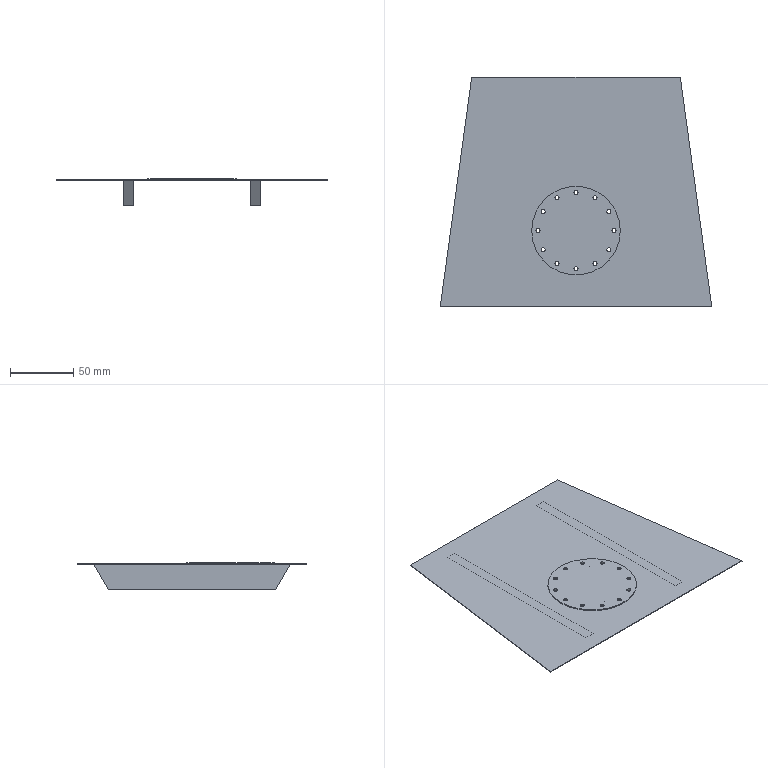Part | SolidWorks | features BaseBody 1 | 1 solid | 46 faces | box 214.2 x 181 x 21.3 mm | volume 65017 mm3 | cylinder 28 | plane 18 | commonest cylinder face diameters 3.2 x24 50 x2 70 x2
STEP:
#1=CARTESIAN_POINT('',(-16.6,85.981,1.3));
#2=VERTEX_POINT('',#1);
#3=CARTESIAN_POINT('',(-13.4,85.981,1.3));
#4=VERTEX_POINT('',#3);
#5=CARTESIAN_POINT('',(-15.,85.981,1.3));
#6=DIRECTION('',(0.,0.,1.));
#7=DIRECTION('',(-1.,0.,0.));
#8=AXIS2_PLACEMENT_3D('',#5,#6,#7);
#9=CIRCLE('',#8,1.6);
#10=EDGE_CURVE('',#2,#4,#9,.T.);
#11=ORIENTED_EDGE('',*,*,#10,.T.);
#12=CARTESIAN_POINT('',(-13.4,85.981,0.));
#13=VERTEX_POINT('',#12);
#14=CARTESIAN_POINT('',(-13.4,85.981,1.3));
#15=DIRECTION('',(0.,0.,-1.));
#16=VECTOR('',#15,1000.);
#17=LINE('',#14,#16);
#18=EDGE_CURVE('',#4,#13,#17,.T.);
#19=ORIENTED_EDGE('',*,*,#18,.T.);
#20=CARTESIAN_POINT('',(-16.6,85.981,0.));
#21=VERTEX_POINT('',#20);
#22=CARTESIAN_POINT('',(-15.,85.981,0.));
#23=DIRECTION('',(0.,0.,-1.));
#24=DIRECTION('',(-1.,0.,0.));
#25=AXIS2_PLACEMENT_3D('',#22,#23,#24);
#26=CIRCLE('',#25,1.6);
#27=EDGE_CURVE('',#13,#21,#26,.T.);
#28=ORIENTED_EDGE('',*,*,#27,.T.);
#29=CARTESIAN_POINT('',(-16.6,85.981,1.3));
#30=DIRECTION('',(0.,0.,-1.));
#31=VECTOR('',#30,1000.);
#32=LINE('',#29,#31);
#33=EDGE_CURVE('',#2,#21,#32,.T.);
#34=ORIENTED_EDGE('',*,*,#33,.F.);
#35=EDGE_LOOP('',(#11,#19,#28,#34));
#36=FACE_OUTER_BOUND('',#35,.T.);
#37=CARTESIAN_POINT('',(-15.,85.981,1.3));
#38=DIRECTION('',(0.,0.,-1.));
#39=DIRECTION('',(-1.,0.,0.));
#40=AXIS2_PLACEMENT_3D('',#37,#38,#39);
#41=CYLINDRICAL_SURFACE('',#40,1.6);
#42=ADVANCED_FACE('',(#36),#41,.F.);
#43=CARTESIAN_POINT('',(-25.,60.,0.5));
#44=VERTEX_POINT('',#43);
#45=CARTESIAN_POINT('',(25.,60.,0.5));
#46=VERTEX_POINT('',#45);
#47=CARTESIAN_POINT('',(0.,60.,0.5));
#48=DIRECTION('',(0.,0.,1.));
#49=DIRECTION('',(-1.,0.,0.));
#50=AXIS2_PLACEMENT_3D('',#47,#48,#49);
#51=CIRCLE('',#50,25.);
#52=EDGE_CURVE('',#44,#46,#51,.T.);
#53=ORIENTED_EDGE('',*,*,#52,.T.);
#54=CARTESIAN_POINT('',(25.,60.,0.));
#55=VERTEX_POINT('',#54);
#56=CARTESIAN_POINT('',(25.,60.,0.5));
#57=DIRECTION('',(0.,0.,-1.));
#58=VECTOR('',#57,1000.);
#59=LINE('',#56,#58);
#60=EDGE_CURVE('',#46,#55,#59,.T.);
#61=ORIENTED_EDGE('',*,*,#60,.T.);
#62=CARTESIAN_POINT('',(-25.,60.,0.));
#63=VERTEX_POINT('',#62);
#64=CARTESIAN_POINT('',(0.,60.,0.));
#65=DIRECTION('',(0.,0.,-1.));
#66=DIRECTION('',(-1.,0.,0.));
#67=AXIS2_PLACEMENT_3D('',#64,#65,#66);
#68=CIRCLE('',#67,25.);
#69=EDGE_CURVE('',#55,#63,#68,.T.);
#70=ORIENTED_EDGE('',*,*,#69,.T.);
#71=CARTESIAN_POINT('',(-25.,60.,0.5));
#72=DIRECTION('',(0.,0.,-1.));
#73=VECTOR('',#72,1000.);
#74=LINE('',#71,#73);
#75=EDGE_CURVE('',#44,#63,#74,.T.);
#76=ORIENTED_EDGE('',*,*,#75,.F.);
#77=EDGE_LOOP('',(#53,#61,#70,#76));
#78=FACE_OUTER_BOUND('',#77,.T.);
#79=CARTESIAN_POINT('',(0.,60.,0.5));
#80=DIRECTION('',(0.,0.,-1.));
#81=DIRECTION('',(-1.,0.,0.));
#82=AXIS2_PLACEMENT_3D('',#79,#80,#81);
#83=CYLINDRICAL_SURFACE('',#82,25.);
#84=ADVANCED_FACE('',(#78),#83,.F.);
#85=CARTESIAN_POINT('',(-24.381,45.,1.3));
#86=VERTEX_POINT('',#85);
#87=CARTESIAN_POINT('',(-27.581,45.,1.3));
#88=VERTEX_POINT('',#87);
#89=CARTESIAN_POINT('',(-25.981,45.,1.3));
#90=DIRECTION('',(0.,0.,-1.));
#91=DIRECTION('',(-1.,0.,0.));
#92=AXIS2_PLACEMENT_3D('',#89,#90,#91);
#93=CIRCLE('',#92,1.6);
#94=EDGE_CURVE('',#86,#88,#93,.T.);
#95=ORIENTED_EDGE('',*,*,#94,.F.);
#96=CARTESIAN_POINT('',(-24.381,45.,0.));
#97=VERTEX_POINT('',#96);
#98=CARTESIAN_POINT('',(-24.381,45.,1.3));
#99=DIRECTION('',(0.,0.,-1.));
#100=VECTOR('',#99,1000.);
#101=LINE('',#98,#100);
#102=EDGE_CURVE('',#86,#97,#101,.T.);
#103=ORIENTED_EDGE('',*,*,#102,.T.);
#104=CARTESIAN_POINT('',(-27.581,45.,0.));
#105=VERTEX_POINT('',#104);
#106=CARTESIAN_POINT('',(-25.981,45.,0.));
#107=DIRECTION('',(0.,0.,-1.));
#108=DIRECTION('',(-1.,0.,0.));
#109=AXIS2_PLACEMENT_3D('',#106,#107,#108);
#110=CIRCLE('',#109,1.6);
#111=EDGE_CURVE('',#97,#105,#110,.T.);
#112=ORIENTED_EDGE('',*,*,#111,.T.);
#113=CARTESIAN_POINT('',(-27.581,45.,1.3));
#114=DIRECTION('',(0.,0.,-1.));
#115=VECTOR('',#114,1000.);
#116=LINE('',#113,#115);
#117=EDGE_CURVE('',#88,#105,#116,.T.);
#118=ORIENTED_EDGE('',*,*,#117,.F.);
#119=EDGE_LOOP('',(#95,#103,#112,#118));
#120=FACE_OUTER_BOUND('',#119,.T.);
#121=CARTESIAN_POINT('',(-25.981,45.,1.3));
#122=DIRECTION('',(0.,0.,-1.));
#123=DIRECTION('',(-1.,0.,0.));
#124=AXIS2_PLACEMENT_3D('',#121,#122,#123);
#125=CYLINDRICAL_SURFACE('',#124,1.6);
#126=ADVANCED_FACE('',(#120),#125,.F.);
#127=CARTESIAN_POINT('',(-13.4,34.019,1.3));
#128=VERTEX_POINT('',#127);
#129=CARTESIAN_POINT('',(-16.6,34.019,1.3));
#130=VERTEX_POINT('',#129);
#131=CARTESIAN_POINT('',(-15.,34.019,1.3));
#132=DIRECTION('',(0.,0.,-1.));
#133=DIRECTION('',(-1.,0.,0.));
#134=AXIS2_PLACEMENT_3D('',#131,#132,#133);
#135=CIRCLE('',#134,1.6);
#136=EDGE_CURVE('',#128,#130,#135,.T.);
#137=ORIENTED_EDGE('',*,*,#136,.F.);
#138=CARTESIAN_POINT('',(-13.4,34.019,0.));
#139=VERTEX_POINT('',#138);
#140=CARTESIAN_POINT('',(-13.4,34.019,1.3));
#141=DIRECTION('',(0.,0.,-1.));
#142=VECTOR('',#141,1000.);
#143=LINE('',#140,#142);
#144=EDGE_CURVE('',#128,#139,#143,.T.);
#145=ORIENTED_EDGE('',*,*,#144,.T.);
#146=CARTESIAN_POINT('',(-16.6,34.019,0.));
#147=VERTEX_POINT('',#146);
#148=CARTESIAN_POINT('',(-15.,34.019,0.));
#149=DIRECTION('',(0.,0.,-1.));
#150=DIRECTION('',(-1.,0.,0.));
#151=AXIS2_PLACEMENT_3D('',#148,#149,#150);
#152=CIRCLE('',#151,1.6);
#153=EDGE_CURVE('',#139,#147,#152,.T.);
#154=ORIENTED_EDGE('',*,*,#153,.T.);
#155=CARTESIAN_POINT('',(-16.6,34.019,1.3));
#156=DIRECTION('',(0.,0.,-1.));
#157=VECTOR('',#156,1000.);
#158=LINE('',#155,#157);
#159=EDGE_CURVE('',#130,#147,#158,.T.);
#160=ORIENTED_EDGE('',*,*,#159,.F.);
#161=EDGE_LOOP('',(#137,#145,#154,#160));
#162=FACE_OUTER_BOUND('',#161,.T.);
#163=CARTESIAN_POINT('',(-15.,34.019,1.3));
#164=DIRECTION('',(0.,0.,-1.));
#165=DIRECTION('',(-1.,0.,0.));
#166=AXIS2_PLACEMENT_3D('',#163,#164,#165);
#167=CYLINDRICAL_SURFACE('',#166,1.6);
#168=ADVANCED_FACE('',(#162),#167,.F.);
#169=CARTESIAN_POINT('',(1.6,30.,1.3));
#170=VERTEX_POINT('',#169);
#171=CARTESIAN_POINT('',(-1.6,30.,1.3));
#172=VERTEX_POINT('',#171);
#173=CARTESIAN_POINT('',(0.,30.,1.3));
#174=DIRECTION('',(0.,0.,-1.));
#175=DIRECTION('',(-1.,0.,0.));
#176=AXIS2_PLACEMENT_3D('',#173,#174,#175);
#177=CIRCLE('',#176,1.6);
#178=EDGE_CURVE('',#170,#172,#177,.T.);
#179=ORIENTED_EDGE('',*,*,#178,.F.);
#180=CARTESIAN_POINT('',(1.6,30.,0.));
#181=VERTEX_POINT('',#180);
#182=CARTESIAN_POINT('',(1.6,30.,1.3));
#183=DIRECTION('',(0.,0.,-1.));
#184=VECTOR('',#183,1000.);
#185=LINE('',#182,#184);
#186=EDGE_CURVE('',#170,#181,#185,.T.);
#187=ORIENTED_EDGE('',*,*,#186,.T.);
#188=CARTESIAN_POINT('',(-1.6,30.,0.));
#189=VERTEX_POINT('',#188);
#190=CARTESIAN_POINT('',(0.,30.,0.));
#191=DIRECTION('',(0.,0.,-1.));
#192=DIRECTION('',(-1.,0.,0.));
#193=AXIS2_PLACEMENT_3D('',#190,#191,#192);
#194=CIRCLE('',#193,1.6);
#195=EDGE_CURVE('',#181,#189,#194,.T.);
#196=ORIENTED_EDGE('',*,*,#195,.T.);
#197=CARTESIAN_POINT('',(-1.6,30.,1.3));
#198=DIRECTION('',(0.,0.,-1.));
#199=VECTOR('',#198,1000.);
#200=LINE('',#197,#199);
#201=EDGE_CURVE('',#172,#189,#200,.T.);
#202=ORIENTED_EDGE('',*,*,#201,.F.);
#203=EDGE_LOOP('',(#179,#187,#196,#202));
#204=FACE_OUTER_BOUND('',#203,.T.);
#205=CARTESIAN_POINT('',(0.,30.,1.3));
#206=DIRECTION('',(0.,0.,-1.));
#207=DIRECTION('',(-1.,0.,0.));
#208=AXIS2_PLACEMENT_3D('',#205,#206,#207);
#209=CYLINDRICAL_SURFACE('',#208,1.6);
#210=ADVANCED_FACE('',(#204),#209,.F.);
#211=CARTESIAN_POINT('',(16.6,34.019,1.3));
#212=VERTEX_POINT('',#211);
#213=CARTESIAN_POINT('',(13.4,34.019,1.3));
#214=VERTEX_POINT('',#213);
#215=CARTESIAN_POINT('',(15.,34.019,1.3));
#216=DIRECTION('',(0.,0.,-1.));
#217=DIRECTION('',(-1.,0.,0.));
#218=AXIS2_PLACEMENT_3D('',#215,#216,#217);
#219=CIRCLE('',#218,1.6);
#220=EDGE_CURVE('',#212,#214,#219,.T.);
#221=ORIENTED_EDGE('',*,*,#220,.F.);
#222=CARTESIAN_POINT('',(16.6,34.019,0.));
#223=VERTEX_POINT('',#222);
#224=CARTESIAN_POINT('',(16.6,34.019,1.3));
#225=DIRECTION('',(0.,0.,-1.));
#226=VECTOR('',#225,1000.);
#227=LINE('',#224,#226);
#228=EDGE_CURVE('',#212,#223,#227,.T.);
#229=ORIENTED_EDGE('',*,*,#228,.T.);
#230=CARTESIAN_POINT('',(13.4,34.019,0.));
#231=VERTEX_POINT('',#230);
#232=CARTESIAN_POINT('',(15.,34.019,0.));
#233=DIRECTION('',(0.,0.,-1.));
#234=DIRECTION('',(-1.,0.,0.));
#235=AXIS2_PLACEMENT_3D('',#232,#233,#234);
#236=CIRCLE('',#235,1.6);
#237=EDGE_CURVE('',#223,#231,#236,.T.);
#238=ORIENTED_EDGE('',*,*,#237,.T.);
#239=CARTESIAN_POINT('',(13.4,34.019,1.3));
#240=DIRECTION('',(0.,0.,-1.));
#241=VECTOR('',#240,1000.);
#242=LINE('',#239,#241);
#243=EDGE_CURVE('',#214,#231,#242,.T.);
#244=ORIENTED_EDGE('',*,*,#243,.F.);
#245=EDGE_LOOP('',(#221,#229,#238,#244));
#246=FACE_OUTER_BOUND('',#245,.T.);
#247=CARTESIAN_POINT('',(15.,34.019,1.3));
#248=DIRECTION('',(0.,0.,-1.));
#249=DIRECTION('',(-1.,0.,0.));
#250=AXIS2_PLACEMENT_3D('',#247,#248,#249);
#251=CYLINDRICAL_SURFACE('',#250,1.6);
#252=ADVANCED_FACE('',(#246),#251,.F.);
#253=CARTESIAN_POINT('',(27.581,45.,1.3));
#254=VERTEX_POINT('',#253);
#255=CARTESIAN_POINT('',(24.381,45.,1.3));
#256=VERTEX_POINT('',#255);
#257=CARTESIAN_POINT('',(25.981,45.,1.3));
#258=DIRECTION('',(0.,0.,-1.));
#259=DIRECTION('',(-1.,0.,0.));
#260=AXIS2_PLACEMENT_3D('',#257,#258,#259);
#261=CIRCLE('',#260,1.6);
#262=EDGE_CURVE('',#254,#256,#261,.T.);
#263=ORIENTED_EDGE('',*,*,#262,.F.);
#264=CARTESIAN_POINT('',(27.581,45.,0.));
#265=VERTEX_POINT('',#264);
#266=CARTESIAN_POINT('',(27.581,45.,1.3));
#267=DIRECTION('',(0.,0.,-1.));
#268=VECTOR('',#267,1000.);
#269=LINE('',#266,#268);
#270=EDGE_CURVE('',#254,#265,#269,.T.);
#271=ORIENTED_EDGE('',*,*,#270,.T.);
#272=CARTESIAN_POINT('',(24.381,45.,0.));
#273=VERTEX_POINT('',#272);
#274=CARTESIAN_POINT('',(25.981,45.,0.));
#275=DIRECTION('',(0.,0.,-1.));
#276=DIRECTION('',(-1.,0.,0.));
#277=AXIS2_PLACEMENT_3D('',#274,#275,#276);
#278=CIRCLE('',#277,1.6);
#279=EDGE_CURVE('',#265,#273,#278,.T.);
#280=ORIENTED_EDGE('',*,*,#279,.T.);
#281=CARTESIAN_POINT('',(24.381,45.,1.3));
#282=DIRECTION('',(0.,0.,-1.));
#283=VECTOR('',#282,1000.);
#284=LINE('',#281,#283);
#285=EDGE_CURVE('',#256,#273,#284,.T.);
#286=ORIENTED_EDGE('',*,*,#285,.F.);
#287=EDGE_LOOP('',(#263,#271,#280,#286));
#288=FACE_OUTER_BOUND('',#287,.T.);
#289=CARTESIAN_POINT('',(25.981,45.,1.3));
#290=DIRECTION('',(0.,0.,-1.));
#291=DIRECTION('',(-1.,0.,0.));
#292=AXIS2_PLACEMENT_3D('',#289,#290,#291);
#293=CYLINDRICAL_SURFACE('',#292,1.6);
#294=ADVANCED_FACE('',(#288),#293,.F.);
#295=CARTESIAN_POINT('',(31.6,60.,1.3));
#296=VERTEX_POINT('',#295);
#297=CARTESIAN_POINT('',(28.4,60.,1.3));
#298=VERTEX_POINT('',#297);
#299=CARTESIAN_POINT('',(30.,60.,1.3));
#300=DIRECTION('',(0.,0.,-1.));
#301=DIRECTION('',(-1.,0.,0.));
#302=AXIS2_PLACEMENT_3D('',#299,#300,#301);
#303=CIRCLE('',#302,1.6);
#304=EDGE_CURVE('',#296,#298,#303,.T.);
#305=ORIENTED_EDGE('',*,*,#304,.F.);
#306=CARTESIAN_POINT('',(31.6,60.,0.));
#307=VERTEX_POINT('',#306);
#308=CARTESIAN_POINT('',(31.6,60.,1.3));
#309=DIRECTION('',(0.,0.,-1.));
#310=VECTOR('',#309,1000.);
#311=LINE('',#308,#310);
#312=EDGE_CURVE('',#296,#307,#311,.T.);
#313=ORIENTED_EDGE('',*,*,#312,.T.);
#314=CARTESIAN_POINT('',(28.4,60.,0.));
#315=VERTEX_POINT('',#314);
#316=CARTESIAN_POINT('',(30.,60.,0.));
#317=DIRECTION('',(0.,0.,-1.));
#318=DIRECTION('',(-1.,0.,0.));
#319=AXIS2_PLACEMENT_3D('',#316,#317,#318);
#320=CIRCLE('',#319,1.6);
#321=EDGE_CURVE('',#307,#315,#320,.T.);
#322=ORIENTED_EDGE('',*,*,#321,.T.);
#323=CARTESIAN_POINT('',(28.4,60.,1.3));
#324=DIRECTION('',(0.,0.,-1.));
#325=VECTOR('',#324,1000.);
#326=LINE('',#323,#325);
#327=EDGE_CURVE('',#298,#315,#326,.T.);
#328=ORIENTED_EDGE('',*,*,#327,.F.);
#329=EDGE_LOOP('',(#305,#313,#322,#328));
#330=FACE_OUTER_BOUND('',#329,.T.);
#331=CARTESIAN_POINT('',(30.,60.,1.3));
#332=DIRECTION('',(0.,0.,-1.));
#333=DIRECTION('',(-1.,0.,0.));
#334=AXIS2_PLACEMENT_3D('',#331,#332,#333);
#335=CYLINDRICAL_SURFACE('',#334,1.6);
#336=ADVANCED_FACE('',(#330),#335,.F.);
#337=CARTESIAN_POINT('',(27.581,75.,1.3));
#338=VERTEX_POINT('',#337);
#339=CARTESIAN_POINT('',(24.381,75.,1.3));
#340=VERTEX_POINT('',#339);
#341=CARTESIAN_POINT('',(25.981,75.,1.3));
#342=DIRECTION('',(0.,0.,-1.));
#343=DIRECTION('',(-1.,0.,0.));
#344=AXIS2_PLACEMENT_3D('',#341,#342,#343);
#345=CIRCLE('',#344,1.6);
#346=EDGE_CURVE('',#338,#340,#345,.T.);
#347=ORIENTED_EDGE('',*,*,#346,.F.);
#348=CARTESIAN_POINT('',(27.581,75.,0.));
#349=VERTEX_POINT('',#348);
#350=CARTESIAN_POINT('',(27.581,75.,1.3));
#351=DIRECTION('',(0.,0.,-1.));
#352=VECTOR('',#351,1000.);
#353=LINE('',#350,#352);
#354=EDGE_CURVE('',#338,#349,#353,.T.);
#355=ORIENTED_EDGE('',*,*,#354,.T.);
#356=CARTESIAN_POINT('',(24.381,75.,0.));
#357=VERTEX_POINT('',#356);
#358=CARTESIAN_POINT('',(25.981,75.,0.));
#359=DIRECTION('',(0.,0.,-1.));
#360=DIRECTION('',(-1.,0.,0.));
#361=AXIS2_PLACEMENT_3D('',#358,#359,#360);
#362=CIRCLE('',#361,1.6);
#363=EDGE_CURVE('',#349,#357,#362,.T.);
#364=ORIENTED_EDGE('',*,*,#363,.T.);
#365=CARTESIAN_POINT('',(24.381,75.,1.3));
#366=DIRECTION('',(0.,0.,-1.));
#367=VECTOR('',#366,1000.);
#368=LINE('',#365,#367);
#369=EDGE_CURVE('',#340,#357,#368,.T.);
#370=ORIENTED_EDGE('',*,*,#369,.F.);
#371=EDGE_LOOP('',(#347,#355,#364,#370));
#372=FACE_OUTER_BOUND('',#371,.T.);
#373=CARTESIAN_POINT('',(25.981,75.,1.3));
#374=DIRECTION('',(0.,0.,-1.));
#375=DIRECTION('',(-1.,0.,0.));
#376=AXIS2_PLACEMENT_3D('',#373,#374,#375);
#377=CYLINDRICAL_SURFACE('',#376,1.6);
#378=ADVANCED_FACE('',(#372),#377,.F.);
#379=CARTESIAN_POINT('',(16.6,85.981,1.3));
#380=VERTEX_POINT('',#379);
#381=CARTESIAN_POINT('',(13.4,85.981,1.3));
#382=VERTEX_POINT('',#381);
#383=CARTESIAN_POINT('',(15.,85.981,1.3));
#384=DIRECTION('',(0.,0.,-1.));
#385=DIRECTION('',(-1.,0.,0.));
#386=AXIS2_PLACEMENT_3D('',#383,#384,#385);
#387=CIRCLE('',#386,1.6);
#388=EDGE_CURVE('',#380,#382,#387,.T.);
#389=ORIENTED_EDGE('',*,*,#388,.F.);
#390=CARTESIAN_POINT('',(16.6,85.981,0.));
#391=VERTEX_POINT('',#390);
#392=CARTESIAN_POINT('',(16.6,85.981,1.3));
#393=DIRECTION('',(0.,0.,-1.));
#394=VECTOR('',#393,1000.);
#395=LINE('',#392,#394);
#396=EDGE_CURVE('',#380,#391,#395,.T.);
#397=ORIENTED_EDGE('',*,*,#396,.T.);
#398=CARTESIAN_POINT('',(13.4,85.981,0.));
#399=VERTEX_POINT('',#398);
#400=CARTESIAN_POINT('',(15.,85.981,0.));
#401=DIRECTION('',(0.,0.,-1.));
#402=DIRECTION('',(-1.,0.,0.));
#403=AXIS2_PLACEMENT_3D('',#400,#401,#402);
#404=CIRCLE('',#403,1.6);
#405=EDGE_CURVE('',#391,#399,#404,.T.);
#406=ORIENTED_EDGE('',*,*,#405,.T.);
#407=CARTESIAN_POINT('',(13.4,85.981,1.3));
#408=DIRECTION('',(0.,0.,-1.));
#409=VECTOR('',#408,1000.);
#410=LINE('',#407,#409);
#411=EDGE_CURVE('',#382,#399,#410,.T.);
#412=ORIENTED_EDGE('',*,*,#411,.F.);
#413=EDGE_LOOP('',(#389,#397,#406,#412));
#414=FACE_OUTER_BOUND('',#413,.T.);
#415=CARTESIAN_POINT('',(15.,85.981,1.3));
#416=DIRECTION('',(0.,0.,-1.));
#417=DIRECTION('',(-1.,0.,0.));
#418=AXIS2_PLACEMENT_3D('',#415,#416,#417);
#419=CYLINDRICAL_SURFACE('',#418,1.6);
#420=ADVANCED_FACE('',(#414),#419,.F.);
#421=CARTESIAN_POINT('',(1.6,90.,1.3));
#422=VERTEX_POINT('',#421);
#423=CARTESIAN_POINT('',(-1.6,90.,1.3));
#424=VERTEX_POINT('',#423);
#425=CARTESIAN_POINT('',(0.,90.,1.3));
#426=DIRECTION('',(0.,0.,-1.));
#427=DIRECTION('',(-1.,0.,0.));
#428=AXIS2_PLACEMENT_3D('',#425,#426,#427);
#429=CIRCLE('',#428,1.6);
#430=EDGE_CURVE('',#422,#424,#429,.T.);
#431=ORIENTED_EDGE('',*,*,#430,.F.);
#432=CARTESIAN_POINT('',(1.6,90.,0.));
#433=VERTEX_POINT('',#432);
#434=CARTESIAN_POINT('',(1.6,90.,1.3));
#435=DIRECTION('',(0.,0.,-1.));
#436=VECTOR('',#435,1000.);
#437=LINE('',#434,#436);
#438=EDGE_CURVE('',#422,#433,#437,.T.);
#439=ORIENTED_EDGE('',*,*,#438,.T.);
#440=CARTESIAN_POINT('',(-1.6,90.,0.));
#441=VERTEX_POINT('',#440);
#442=CARTESIAN_POINT('',(0.,90.,0.));
#443=DIRECTION('',(0.,0.,-1.));
#444=DIRECTION('',(-1.,0.,0.));
#445=AXIS2_PLACEMENT_3D('',#442,#443,#444);
#446=CIRCLE('',#445,1.6);
#447=EDGE_CURVE('',#433,#441,#446,.T.);
#448=ORIENTED_EDGE('',*,*,#447,.T.);
#449=CARTESIAN_POINT('',(-1.6,90.,1.3));
#450=DIRECTION('',(0.,0.,-1.));
#451=VECTOR('',#450,1000.);
#452=LINE('',#449,#451);
#453=EDGE_CURVE('',#424,#441,#452,.T.);
#454=ORIENTED_EDGE('',*,*,#453,.F.);
#455=EDGE_LOOP('',(#431,#439,#448,#454));
#456=FACE_OUTER_BOUND('',#455,.T.);
#457=CARTESIAN_POINT('',(0.,90.,1.3));
#458=DIRECTION('',(0.,0.,-1.));
#459=DIRECTION('',(-1.,0.,0.));
#460=AXIS2_PLACEMENT_3D('',#457,#458,#459);
#461=CYLINDRICAL_SURFACE('',#460,1.6);
#462=ADVANCED_FACE('',(#456),#461,.F.);
#463=CARTESIAN_POINT('',(-24.381,75.,1.3));
#464=VERTEX_POINT('',#463);
#465=CARTESIAN_POINT('',(-27.581,75.,1.3));
#466=VERTEX_POINT('',#465);
#467=CARTESIAN_POINT('',(-25.981,75.,1.3));
#468=DIRECTION('',(0.,0.,-1.));
#469=DIRECTION('',(-1.,0.,0.));
#470=AXIS2_PLACEMENT_3D('',#467,#468,#469);
#471=CIRCLE('',#470,1.6);
#472=EDGE_CURVE('',#464,#466,#471,.T.);
#473=ORIENTED_EDGE('',*,*,#472,.F.);
#474=CARTESIAN_POINT('',(-24.381,75.,0.));
#475=VERTEX_POINT('',#474);
#476=CARTESIAN_POINT('',(-24.381,75.,1.3));
#477=DIRECTION('',(0.,0.,-1.));
#478=VECTOR('',#477,1000.);
#479=LINE('',#476,#478);
#480=EDGE_CURVE('',#464,#475,#479,.T.);
#481=ORIENTED_EDGE('',*,*,#480,.T.);
#482=CARTESIAN_POINT('',(-27.581,75.,0.));
#483=VERTEX_POINT('',#482);
#484=CARTESIAN_POINT('',(-25.981,75.,0.));
#485=DIRECTION('',(0.,0.,-1.));
#486=DIRECTION('',(-1.,0.,0.));
#487=AXIS2_PLACEMENT_3D('',#484,#485,#486);
#488=CIRCLE('',#487,1.6);
#489=EDGE_CURVE('',#475,#483,#488,.T.);
#490=ORIENTED_EDGE('',*,*,#489,.T.);
#491=CARTESIAN_POINT('',(-27.581,75.,1.3));
#492=DIRECTION('',(0.,0.,-1.));
#493=VECTOR('',#492,1000.);
#494=LINE('',#491,#493);
#495=EDGE_CURVE('',#466,#483,#494,.T.);
#496=ORIENTED_EDGE('',*,*,#495,.F.);
#497=EDGE_LOOP('',(#473,#481,#490,#496));
#498=FACE_OUTER_BOUND('',#497,.T.);
#499=CARTESIAN_POINT('',(-25.981,75.,1.3));
#500=DIRECTION('',(0.,0.,-1.));
#501=DIRECTION('',(-1.,0.,0.));
#502=AXIS2_PLACEMENT_3D('',#499,#500,#501);
#503=CYLINDRICAL_SURFACE('',#502,1.6);
#504=ADVANCED_FACE('',(#498),#503,.F.);
#505=CARTESIAN_POINT('',(-28.4,60.,1.3));
#506=VERTEX_POINT('',#505);
#507=CARTESIAN_POINT('',(-31.6,60.,1.3));
#508=VERTEX_POINT('',#507);
#509=CARTESIAN_POINT('',(-30.,60.,1.3));
#510=DIRECTION('',(0.,0.,-1.));
#511=DIRECTION('',(-1.,0.,0.));
#512=AXIS2_PLACEMENT_3D('',#509,#510,#511);
#513=CIRCLE('',#512,1.6);
#514=EDGE_CURVE('',#506,#508,#513,.T.);
#515=ORIENTED_EDGE('',*,*,#514,.F.);
#516=CARTESIAN_POINT('',(-28.4,60.,0.));
#517=VERTEX_POINT('',#516);
#518=CARTESIAN_POINT('',(-28.4,60.,1.3));
#519=DIRECTION('',(0.,0.,-1.));
#520=VECTOR('',#519,1000.);
#521=LINE('',#518,#520);
#522=EDGE_CURVE('',#506,#517,#521,.T.);
#523=ORIENTED_EDGE('',*,*,#522,.T.);
#524=CARTESIAN_POINT('',(-31.6,60.,0.));
#525=VERTEX_POINT('',#524);
#526=CARTESIAN_POINT('',(-30.,60.,0.));
#527=DIRECTION('',(0.,0.,-1.));
#528=DIRECTION('',(-1.,0.,0.));
#529=AXIS2_PLACEMENT_3D('',#526,#527,#528);
#530=CIRCLE('',#529,1.6);
#531=EDGE_CURVE('',#517,#525,#530,.T.);
#532=ORIENTED_EDGE('',*,*,#531,.T.);
#533=CARTESIAN_POINT('',(-31.6,60.,1.3));
#534=DIRECTION('',(0.,0.,-1.));
#535=VECTOR('',#534,1000.);
#536=LINE('',#533,#535);
#537=EDGE_CURVE('',#508,#525,#536,.T.);
#538=ORIENTED_EDGE('',*,*,#537,.F.);
#539=EDGE_LOOP('',(#515,#523,#532,#538));
#540=FACE_OUTER_BOUND('',#539,.T.);
#541=CARTESIAN_POINT('',(-30.,60.,1.3));
#542=DIRECTION('',(0.,0.,-1.));
#543=DIRECTION('',(-1.,0.,0.));
#544=AXIS2_PLACEMENT_3D('',#541,#542,#543);
#545=CYLINDRICAL_SURFACE('',#544,1.6);
#546=ADVANCED_FACE('',(#540),#545,.F.);
#547=CARTESIAN_POINT('',(35.,60.,1.3));
#548=VERTEX_POINT('',#547);
#549=CARTESIAN_POINT('',(-35.,60.,1.3));
#550=VERTEX_POINT('',#549);
#551=CARTESIAN_POINT('',(0.,60.,1.3));
#552=DIRECTION('',(0.,0.,1.));
#553=DIRECTION('',(-1.,0.,0.));
#554=AXIS2_PLACEMENT_3D('',#551,#552,#553);
#555=CIRCLE('',#554,35.);
#556=EDGE_CURVE('',#548,#550,#555,.T.);
#557=ORIENTED_EDGE('',*,*,#556,.F.);
#558=CARTESIAN_POINT('',(35.,60.,0.5));
#559=VERTEX_POINT('',#558);
#560=CARTESIAN_POINT('',(35.,60.,1.3));
#561=DIRECTION('',(0.,0.,-1.));
#562=VECTOR('',#561,1000.);
#563=LINE('',#560,#562);
#564=EDGE_CURVE('',#548,#559,#563,.T.);
#565=ORIENTED_EDGE('',*,*,#564,.T.);
#566=CARTESIAN_POINT('',(-35.,60.,0.5));
#567=VERTEX_POINT('',#566);
#568=CARTESIAN_POINT('',(0.,60.,0.5));
#569=DIRECTION('',(0.,0.,-1.));
#570=DIRECTION('',(-1.,0.,0.));
#571=AXIS2_PLACEMENT_3D('',#568,#569,#570);
#572=CIRCLE('',#571,35.);
#573=EDGE_CURVE('',#567,#559,#572,.T.);
#574=ORIENTED_EDGE('',*,*,#573,.F.);
#575=CARTESIAN_POINT('',(-35.,60.,1.3));
#576=DIRECTION('',(0.,0.,-1.));
#577=VECTOR('',#576,1000.);
#578=LINE('',#575,#577);
#579=EDGE_CURVE('',#550,#567,#578,.T.);
#580=ORIENTED_EDGE('',*,*,#579,.F.);
#581=EDGE_LOOP('',(#557,#565,#574,#580));
#582=FACE_OUTER_BOUND('',#581,.T.);
#583=CARTESIAN_POINT('',(0.,60.,1.3));
#584=DIRECTION('',(0.,0.,-1.));
#585=DIRECTION('',(-1.,0.,0.));
#586=AXIS2_PLACEMENT_3D('',#583,#584,#585);
#587=CYLINDRICAL_SURFACE('',#586,35.);
#588=ADVANCED_FACE('',(#582),#587,.T.);
#589=ORIENTED_EDGE('',*,*,#18,.F.);
#590=CARTESIAN_POINT('',(-15.,85.981,1.3));
#591=DIRECTION('',(0.,0.,1.));
#592=DIRECTION('',(-1.,0.,0.));
#593=AXIS2_PLACEMENT_3D('',#590,#591,#592);
#594=CIRCLE('',#593,1.6);
#595=EDGE_CURVE('',#4,#2,#594,.T.);
#596=ORIENTED_EDGE('',*,*,#595,.T.);
#597=ORIENTED_EDGE('',*,*,#33,.T.);
#598=CARTESIAN_POINT('',(-15.,85.981,0.));
#599=DIRECTION('',(0.,0.,-1.));
#600=DIRECTION('',(-1.,0.,0.));
#601=AXIS2_PLACEMENT_3D('',#598,#599,#600);
#602=CIRCLE('',#601,1.6);
#603=EDGE_CURVE('',#21,#13,#602,.T.);
#604=ORIENTED_EDGE('',*,*,#603,.T.);
#605=EDGE_LOOP('',(#589,#596,#597,#604));
#606=FACE_OUTER_BOUND('',#605,.T.);
#607=CARTESIAN_POINT('',(-15.,85.981,1.3));
#608=DIRECTION('',(0.,0.,-1.));
#609=DIRECTION('',(-1.,0.,0.));
#610=AXIS2_PLACEMENT_3D('',#607,#608,#609);
#611=CYLINDRICAL_SURFACE('',#610,1.6);
#612=ADVANCED_FACE('',(#606),#611,.F.);
#613=CARTESIAN_POINT('',(0.,60.,0.));
#614=DIRECTION('',(0.,0.,-1.));
#615=DIRECTION('',(-1.,0.,0.));
#616=AXIS2_PLACEMENT_3D('',#613,#614,#615);
#617=CIRCLE('',#616,25.);
#618=EDGE_CURVE('',#63,#55,#617,.T.);
#619=ORIENTED_EDGE('',*,*,#618,.F.);
#620=ORIENTED_EDGE('',*,*,#69,.F.);
#621=EDGE_LOOP('',(#619,#620));
#622=FACE_BOUND('',#621,.T.);
#623=CARTESIAN_POINT('',(-25.981,45.,0.));
#624=DIRECTION('',(0.,0.,-1.));
#625=DIRECTION('',(-1.,0.,0.));
#626=AXIS2_PLACEMENT_3D('',#623,#624,#625);
#627=CIRCLE('',#626,1.6);
#628=EDGE_CURVE('',#105,#97,#627,.T.);
#629=ORIENTED_EDGE('',*,*,#628,.F.);
#630=ORIENTED_EDGE('',*,*,#111,.F.);
#631=EDGE_LOOP('',(#629,#630));
#632=FACE_BOUND('',#631,.T.);
#633=CARTESIAN_POINT('',(-15.,34.019,0.));
#634=DIRECTION('',(0.,0.,-1.));
#635=DIRECTION('',(-1.,0.,0.));
#636=AXIS2_PLACEMENT_3D('',#633,#634,#635);
#637=CIRCLE('',#636,1.6);
#638=EDGE_CURVE('',#147,#139,#637,.T.);
#639=ORIENTED_EDGE('',*,*,#638,.F.);
#640=ORIENTED_EDGE('',*,*,#153,.F.);
#641=EDGE_LOOP('',(#639,#640));
#642=FACE_BOUND('',#641,.T.);
#643=CARTESIAN_POINT('',(0.,30.,0.));
#644=DIRECTION('',(0.,0.,-1.));
#645=DIRECTION('',(-1.,0.,0.));
#646=AXIS2_PLACEMENT_3D('',#643,#644,#645);
#647=CIRCLE('',#646,1.6);
#648=EDGE_CURVE('',#189,#181,#647,.T.);
#649=ORIENTED_EDGE('',*,*,#648,.F.);
#650=ORIENTED_EDGE('',*,*,#195,.F.);
#651=EDGE_LOOP('',(#649,#650));
#652=FACE_BOUND('',#651,.T.);
#653=CARTESIAN_POINT('',(15.,34.019,0.));
#654=DIRECTION('',(0.,0.,-1.));
#655=DIRECTION('',(-1.,0.,0.));
#656=AXIS2_PLACEMENT_3D('',#653,#654,#655);
#657=CIRCLE('',#656,1.6);
#658=EDGE_CURVE('',#231,#223,#657,.T.);
#659=ORIENTED_EDGE('',*,*,#658,.F.);
#660=ORIENTED_EDGE('',*,*,#237,.F.);
#661=EDGE_LOOP('',(#659,#660));
#662=FACE_BOUND('',#661,.T.);
#663=CARTESIAN_POINT('',(25.981,45.,0.));
#664=DIRECTION('',(0.,0.,-1.));
#665=DIRECTION('',(-1.,0.,0.));
#666=AXIS2_PLACEMENT_3D('',#663,#664,#665);
#667=CIRCLE('',#666,1.6);
#668=EDGE_CURVE('',#273,#265,#667,.T.);
#669=ORIENTED_EDGE('',*,*,#668,.F.);
#670=ORIENTED_EDGE('',*,*,#279,.F.);
#671=EDGE_LOOP('',(#669,#670));
#672=FACE_BOUND('',#671,.T.);
#673=CARTESIAN_POINT('',(30.,60.,0.));
#674=DIRECTION('',(0.,0.,-1.));
#675=DIRECTION('',(-1.,0.,0.));
#676=AXIS2_PLACEMENT_3D('',#673,#674,#675);
#677=CIRCLE('',#676,1.6);
#678=EDGE_CURVE('',#315,#307,#677,.T.);
#679=ORIENTED_EDGE('',*,*,#678,.F.);
#680=ORIENTED_EDGE('',*,*,#321,.F.);
#681=EDGE_LOOP('',(#679,#680));
#682=FACE_BOUND('',#681,.T.);
#683=CARTESIAN_POINT('',(25.981,75.,0.));
#684=DIRECTION('',(0.,0.,-1.));
#685=DIRECTION('',(-1.,0.,0.));
#686=AXIS2_PLACEMENT_3D('',#683,#684,#685);
#687=CIRCLE('',#686,1.6);
#688=EDGE_CURVE('',#357,#349,#687,.T.);
#689=ORIENTED_EDGE('',*,*,#688,.F.);
#690=ORIENTED_EDGE('',*,*,#363,.F.);
#691=EDGE_LOOP('',(#689,#690));
#692=FACE_BOUND('',#691,.T.);
#693=CARTESIAN_POINT('',(15.,85.981,0.));
#694=DIRECTION('',(0.,0.,-1.));
#695=DIRECTION('',(-1.,0.,0.));
#696=AXIS2_PLACEMENT_3D('',#693,#694,#695);
#697=CIRCLE('',#696,1.6);
#698=EDGE_CURVE('',#399,#391,#697,.T.);
#699=ORIENTED_EDGE('',*,*,#698,.F.);
#700=ORIENTED_EDGE('',*,*,#405,.F.);
#701=EDGE_LOOP('',(#699,#700));
#702=FACE_BOUND('',#701,.T.);
#703=CARTESIAN_POINT('',(0.,90.,0.));
#704=DIRECTION('',(0.,0.,-1.));
#705=DIRECTION('',(-1.,0.,0.));
#706=AXIS2_PLACEMENT_3D('',#703,#704,#705);
#707=CIRCLE('',#706,1.6);
#708=EDGE_CURVE('',#441,#433,#707,.T.);
#709=ORIENTED_EDGE('',*,*,#708,.F.);
#710=ORIENTED_EDGE('',*,*,#447,.F.);
#711=EDGE_LOOP('',(#709,#710));
#712=FACE_BOUND('',#711,.T.);
#713=ORIENTED_EDGE('',*,*,#603,.F.);
#714=ORIENTED_EDGE('',*,*,#27,.F.);
#715=EDGE_LOOP('',(#713,#714));
#716=FACE_BOUND('',#715,.T.);
#717=CARTESIAN_POINT('',(-25.981,75.,0.));
#718=DIRECTION('',(0.,0.,-1.));
#719=DIRECTION('',(-1.,0.,0.));
#720=AXIS2_PLACEMENT_3D('',#717,#718,#719);
#721=CIRCLE('',#720,1.6);
#722=EDGE_CURVE('',#483,#475,#721,.T.);
#723=ORIENTED_EDGE('',*,*,#722,.F.);
#724=ORIENTED_EDGE('',*,*,#489,.F.);
#725=EDGE_LOOP('',(#723,#724));
#726=FACE_BOUND('',#725,.T.);
#727=CARTESIAN_POINT('',(-30.,60.,0.));
#728=DIRECTION('',(0.,0.,-1.));
#729=DIRECTION('',(-1.,0.,0.));
#730=AXIS2_PLACEMENT_3D('',#727,#728,#729);
#731=CIRCLE('',#730,1.6);
#732=EDGE_CURVE('',#525,#517,#731,.T.);
#733=ORIENTED_EDGE('',*,*,#732,.F.);
#734=ORIENTED_EDGE('',*,*,#531,.F.);
#735=EDGE_LOOP('',(#733,#734));
#736=FACE_BOUND('',#735,.T.);
#737=CARTESIAN_POINT('',(46.,13.,0.000000008));
#738=VERTEX_POINT('',#737);
#739=CARTESIAN_POINT('',(46.,168.,0.));
#740=VERTEX_POINT('',#739);
#741=CARTESIAN_POINT('',(46.,90.5,0.));
#742=DIRECTION('',(0.,1.,0.));
#743=VECTOR('',#742,1000.);
#744=LINE('',#741,#743);
#745=EDGE_CURVE('',#738,#740,#744,.T.);
#746=ORIENTED_EDGE('',*,*,#745,.F.);
#747=CARTESIAN_POINT('',(54.,13.,0.));
#748=VERTEX_POINT('',#747);
#749=CARTESIAN_POINT('',(0.,13.,0.));
#750=DIRECTION('',(-1.,0.,0.));
#751=VECTOR('',#750,1000.);
#752=LINE('',#749,#751);
#753=EDGE_CURVE('',#748,#738,#752,.T.);
#754=ORIENTED_EDGE('',*,*,#753,.F.);
#755=CARTESIAN_POINT('',(54.,168.,0.));
#756=VERTEX_POINT('',#755);
#757=CARTESIAN_POINT('',(54.,90.5,0.));
#758=DIRECTION('',(0.,-1.,0.));
#759=VECTOR('',#758,1000.);
#760=LINE('',#757,#759);
#761=EDGE_CURVE('',#756,#748,#760,.T.);
#762=ORIENTED_EDGE('',*,*,#761,.F.);
#763=CARTESIAN_POINT('',(0.,168.,0.));
#764=DIRECTION('',(1.,0.,0.));
#765=VECTOR('',#764,1000.);
#766=LINE('',#763,#765);
#767=EDGE_CURVE('',#740,#756,#766,.T.);
#768=ORIENTED_EDGE('',*,*,#767,.F.);
#769=EDGE_LOOP('',(#746,#754,#762,#768));
#770=FACE_BOUND('',#769,.T.);
#771=CARTESIAN_POINT('',(-46.,168.,0.000000008));
#772=VERTEX_POINT('',#771);
#773=CARTESIAN_POINT('',(-46.,13.,0.));
#774=VERTEX_POINT('',#773);
#775=CARTESIAN_POINT('',(-46.,90.5,0.));
#776=DIRECTION('',(0.,-1.,0.));
#777=VECTOR('',#776,1000.);
#778=LINE('',#775,#777);
#779=EDGE_CURVE('',#772,#774,#778,.T.);
#780=ORIENTED_EDGE('',*,*,#779,.F.);
#781=CARTESIAN_POINT('',(-54.,168.,0.));
#782=VERTEX_POINT('',#781);
#783=CARTESIAN_POINT('',(0.,168.,0.));
#784=DIRECTION('',(1.,0.,0.));
#785=VECTOR('',#784,1000.);
#786=LINE('',#783,#785);
#787=EDGE_CURVE('',#782,#772,#786,.T.);
#788=ORIENTED_EDGE('',*,*,#787,.F.);
#789=CARTESIAN_POINT('',(-54.,13.,0.));
#790=VERTEX_POINT('',#789);
#791=CARTESIAN_POINT('',(-54.,90.5,0.));
#792=DIRECTION('',(0.,1.,0.));
#793=VECTOR('',#792,1000.);
#794=LINE('',#791,#793);
#795=EDGE_CURVE('',#790,#782,#794,.T.);
#796=ORIENTED_EDGE('',*,*,#795,.F.);
#797=CARTESIAN_POINT('',(0.,13.,0.));
#798=DIRECTION('',(-1.,0.,0.));
#799=VECTOR('',#798,1000.);
#800=LINE('',#797,#799);
#801=EDGE_CURVE('',#774,#790,#800,.T.);
#802=ORIENTED_EDGE('',*,*,#801,.F.);
#803=EDGE_LOOP('',(#780,#788,#796,#802));
#804=FACE_BOUND('',#803,.T.);
#805=CARTESIAN_POINT('',(-82.3,181.,0.));
#806=VERTEX_POINT('',#805);
#807=CARTESIAN_POINT('',(-107.1,0.,0.));
#808=VERTEX_POINT('',#807);
#809=CARTESIAN_POINT('',(-107.1,0.,0.));
#810=DIRECTION('',(-0.1357,-0.9907,0.));
#811=VECTOR('',#810,1000.);
#812=LINE('',#809,#811);
#813=EDGE_CURVE('',#806,#808,#812,.T.);
#814=ORIENTED_EDGE('',*,*,#813,.F.);
#815=CARTESIAN_POINT('',(82.3,181.,0.));
#816=VERTEX_POINT('',#815);
#817=CARTESIAN_POINT('',(0.,181.,0.));
#818=DIRECTION('',(-1.,0.,0.));
#819=VECTOR('',#818,1000.);
#820=LINE('',#817,#819);
#821=EDGE_CURVE('',#816,#806,#820,.T.);
#822=ORIENTED_EDGE('',*,*,#821,.F.);
#823=CARTESIAN_POINT('',(107.1,0.,0.));
#824=VERTEX_POINT('',#823);
#825=CARTESIAN_POINT('',(82.3,181.,0.));
#826=DIRECTION('',(-0.1357,0.9907,0.));
#827=VECTOR('',#826,1000.);
#828=LINE('',#825,#827);
#829=EDGE_CURVE('',#824,#816,#828,.T.);
#830=ORIENTED_EDGE('',*,*,#829,.F.);
#831=CARTESIAN_POINT('',(0.,0.,0.));
#832=DIRECTION('',(1.,0.,0.));
#833=VECTOR('',#832,1000.);
#834=LINE('',#831,#833);
#835=EDGE_CURVE('',#808,#824,#834,.T.);
#836=ORIENTED_EDGE('',*,*,#835,.F.);
#837=EDGE_LOOP('',(#814,#822,#830,#836));
#838=FACE_OUTER_BOUND('',#837,.T.);
#839=CARTESIAN_POINT('',(-108.385,0.,0.));
#840=DIRECTION('',(0.,0.,1.));
#841=DIRECTION('',(1.,0.,0.));
#842=AXIS2_PLACEMENT_3D('',#839,#840,#841);
#843=PLANE('',#842);
#844=ADVANCED_FACE('',(#622,#632,#642,#652,#662,#672,#682,#692,#702,#712,#716,#726,#736,#770,#804,#838),#843,.F.);
#845=ORIENTED_EDGE('',*,*,#10,.F.);
#846=ORIENTED_EDGE('',*,*,#595,.F.);
#847=EDGE_LOOP('',(#845,#846));
#848=FACE_BOUND('',#847,.T.);
#849=CARTESIAN_POINT('',(-30.,60.,1.3));
#850=DIRECTION('',(0.,0.,-1.));
#851=DIRECTION('',(-1.,0.,0.));
#852=AXIS2_PLACEMENT_3D('',#849,#850,#851);
#853=CIRCLE('',#852,1.6);
#854=EDGE_CURVE('',#508,#506,#853,.T.);
#855=ORIENTED_EDGE('',*,*,#854,.T.);
#856=ORIENTED_EDGE('',*,*,#514,.T.);
#857=EDGE_LOOP('',(#855,#856));
#858=FACE_BOUND('',#857,.T.);
#859=CARTESIAN_POINT('',(-15.,34.019,1.3));
#860=DIRECTION('',(0.,0.,-1.));
#861=DIRECTION('',(-1.,0.,0.));
#862=AXIS2_PLACEMENT_3D('',#859,#860,#861);
#863=CIRCLE('',#862,1.6);
#864=EDGE_CURVE('',#130,#128,#863,.T.);
#865=ORIENTED_EDGE('',*,*,#864,.T.);
#866=ORIENTED_EDGE('',*,*,#136,.T.);
#867=EDGE_LOOP('',(#865,#866));
#868=FACE_BOUND('',#867,.T.);
#869=CARTESIAN_POINT('',(15.,34.019,1.3));
#870=DIRECTION('',(0.,0.,-1.));
#871=DIRECTION('',(-1.,0.,0.));
#872=AXIS2_PLACEMENT_3D('',#869,#870,#871);
#873=CIRCLE('',#872,1.6);
#874=EDGE_CURVE('',#214,#212,#873,.T.);
#875=ORIENTED_EDGE('',*,*,#874,.T.);
#876=ORIENTED_EDGE('',*,*,#220,.T.);
#877=EDGE_LOOP('',(#875,#876));
#878=FACE_BOUND('',#877,.T.);
#879=CARTESIAN_POINT('',(30.,60.,1.3));
#880=DIRECTION('',(0.,0.,-1.));
#881=DIRECTION('',(-1.,0.,0.));
#882=AXIS2_PLACEMENT_3D('',#879,#880,#881);
#883=CIRCLE('',#882,1.6);
#884=EDGE_CURVE('',#298,#296,#883,.T.);
#885=ORIENTED_EDGE('',*,*,#884,.T.);
#886=ORIENTED_EDGE('',*,*,#304,.T.);
#887=EDGE_LOOP('',(#885,#886));
#888=FACE_BOUND('',#887,.T.);
#889=CARTESIAN_POINT('',(15.,85.981,1.3));
#890=DIRECTION('',(0.,0.,-1.));
#891=DIRECTION('',(-1.,0.,0.));
#892=AXIS2_PLACEMENT_3D('',#889,#890,#891);
#893=CIRCLE('',#892,1.6);
#894=EDGE_CURVE('',#382,#380,#893,.T.);
#895=ORIENTED_EDGE('',*,*,#894,.T.);
#896=ORIENTED_EDGE('',*,*,#388,.T.);
#897=EDGE_LOOP('',(#895,#896));
#898=FACE_BOUND('',#897,.T.);
#899=CARTESIAN_POINT('',(0.,90.,1.3));
#900=DIRECTION('',(0.,0.,-1.));
#901=DIRECTION('',(-1.,0.,0.));
#902=AXIS2_PLACEMENT_3D('',#899,#900,#901);
#903=CIRCLE('',#902,1.6);
#904=EDGE_CURVE('',#424,#422,#903,.T.);
#905=ORIENTED_EDGE('',*,*,#904,.T.);
#906=ORIENTED_EDGE('',*,*,#430,.T.);
#907=EDGE_LOOP('',(#905,#906));
#908=FACE_BOUND('',#907,.T.);
#909=CARTESIAN_POINT('',(25.981,75.,1.3));
#910=DIRECTION('',(0.,0.,-1.));
#911=DIRECTION('',(-1.,0.,0.));
#912=AXIS2_PLACEMENT_3D('',#909,#910,#911);
#913=CIRCLE('',#912,1.6);
#914=EDGE_CURVE('',#340,#338,#913,.T.);
#915=ORIENTED_EDGE('',*,*,#914,.T.);
#916=ORIENTED_EDGE('',*,*,#346,.T.);
#917=EDGE_LOOP('',(#915,#916));
#918=FACE_BOUND('',#917,.T.);
#919=CARTESIAN_POINT('',(25.981,45.,1.3));
#920=DIRECTION('',(0.,0.,-1.));
#921=DIRECTION('',(-1.,0.,0.));
#922=AXIS2_PLACEMENT_3D('',#919,#920,#921);
#923=CIRCLE('',#922,1.6);
#924=EDGE_CURVE('',#256,#254,#923,.T.);
#925=ORIENTED_EDGE('',*,*,#924,.T.);
#926=ORIENTED_EDGE('',*,*,#262,.T.);
#927=EDGE_LOOP('',(#925,#926));
#928=FACE_BOUND('',#927,.T.);
#929=CARTESIAN_POINT('',(0.,30.,1.3));
#930=DIRECTION('',(0.,0.,-1.));
#931=DIRECTION('',(-1.,0.,0.));
#932=AXIS2_PLACEMENT_3D('',#929,#930,#931);
#933=CIRCLE('',#932,1.6);
#934=EDGE_CURVE('',#172,#170,#933,.T.);
#935=ORIENTED_EDGE('',*,*,#934,.T.);
#936=ORIENTED_EDGE('',*,*,#178,.T.);
#937=EDGE_LOOP('',(#935,#936));
#938=FACE_BOUND('',#937,.T.);
#939=CARTESIAN_POINT('',(-25.981,45.,1.3));
#940=DIRECTION('',(0.,0.,-1.));
#941=DIRECTION('',(-1.,0.,0.));
#942=AXIS2_PLACEMENT_3D('',#939,#940,#941);
#943=CIRCLE('',#942,1.6);
#944=EDGE_CURVE('',#88,#86,#943,.T.);
#945=ORIENTED_EDGE('',*,*,#944,.T.);
#946=ORIENTED_EDGE('',*,*,#94,.T.);
#947=EDGE_LOOP('',(#945,#946));
#948=FACE_BOUND('',#947,.T.);
#949=CARTESIAN_POINT('',(-25.981,75.,1.3));
#950=DIRECTION('',(0.,0.,-1.));
#951=DIRECTION('',(-1.,0.,0.));
#952=AXIS2_PLACEMENT_3D('',#949,#950,#951);
#953=CIRCLE('',#952,1.6);
#954=EDGE_CURVE('',#466,#464,#953,.T.);
#955=ORIENTED_EDGE('',*,*,#954,.T.);
#956=ORIENTED_EDGE('',*,*,#472,.T.);
#957=EDGE_LOOP('',(#955,#956));
#958=FACE_BOUND('',#957,.T.);
#959=CARTESIAN_POINT('',(0.,60.,1.3));
#960=DIRECTION('',(0.,0.,1.));
#961=DIRECTION('',(-1.,0.,0.));
#962=AXIS2_PLACEMENT_3D('',#959,#960,#961);
#963=CIRCLE('',#962,35.);
#964=EDGE_CURVE('',#550,#548,#963,.T.);
#965=ORIENTED_EDGE('',*,*,#964,.T.);
#966=ORIENTED_EDGE('',*,*,#556,.T.);
#967=EDGE_LOOP('',(#965,#966));
#968=FACE_OUTER_BOUND('',#967,.T.);
#969=CARTESIAN_POINT('',(-35.42,24.58,1.3));
#970=DIRECTION('',(0.,0.,1.));
#971=DIRECTION('',(1.,0.,0.));
#972=AXIS2_PLACEMENT_3D('',#969,#970,#971);
#973=PLANE('',#972);
#974=ADVANCED_FACE('',(#848,#858,#868,#878,#888,#898,#908,#918,#928,#938,#948,#958,#968),#973,.T.);
#975=ORIENTED_EDGE('',*,*,#60,.F.);
#976=CARTESIAN_POINT('',(0.,60.,0.5));
#977=DIRECTION('',(0.,0.,1.));
#978=DIRECTION('',(-1.,0.,0.));
#979=AXIS2_PLACEMENT_3D('',#976,#977,#978);
#980=CIRCLE('',#979,25.);
#981=EDGE_CURVE('',#46,#44,#980,.T.);
#982=ORIENTED_EDGE('',*,*,#981,.T.);
#983=ORIENTED_EDGE('',*,*,#75,.T.);
#984=ORIENTED_EDGE('',*,*,#618,.T.);
#985=EDGE_LOOP('',(#975,#982,#983,#984));
#986=FACE_OUTER_BOUND('',#985,.T.);
#987=CARTESIAN_POINT('',(0.,60.,0.5));
#988=DIRECTION('',(0.,0.,-1.));
#989=DIRECTION('',(-1.,0.,0.));
#990=AXIS2_PLACEMENT_3D('',#987,#988,#989);
#991=CYLINDRICAL_SURFACE('',#990,25.);
#992=ADVANCED_FACE('',(#986),#991,.F.);
#993=ORIENTED_EDGE('',*,*,#102,.F.);
#994=ORIENTED_EDGE('',*,*,#944,.F.);
#995=ORIENTED_EDGE('',*,*,#117,.T.);
#996=ORIENTED_EDGE('',*,*,#628,.T.);
#997=EDGE_LOOP('',(#993,#994,#995,#996));
#998=FACE_OUTER_BOUND('',#997,.T.);
#999=CARTESIAN_POINT('',(-25.981,45.,1.3));
#1000=DIRECTION('',(0.,0.,-1.));
#1001=DIRECTION('',(-1.,0.,0.));
#1002=AXIS2_PLACEMENT_3D('',#999,#1000,#1001);
#1003=CYLINDRICAL_SURFACE('',#1002,1.6);
#1004=ADVANCED_FACE('',(#998),#1003,.F.);
#1005=ORIENTED_EDGE('',*,*,#144,.F.);
#1006=ORIENTED_EDGE('',*,*,#864,.F.);
#1007=ORIENTED_EDGE('',*,*,#159,.T.);
#1008=ORIENTED_EDGE('',*,*,#638,.T.);
#1009=EDGE_LOOP('',(#1005,#1006,#1007,#1008));
#1010=FACE_OUTER_BOUND('',#1009,.T.);
#1011=CARTESIAN_POINT('',(-15.,34.019,1.3));
#1012=DIRECTION('',(0.,0.,-1.));
#1013=DIRECTION('',(-1.,0.,0.));
#1014=AXIS2_PLACEMENT_3D('',#1011,#1012,#1013);
#1015=CYLINDRICAL_SURFACE('',#1014,1.6);
#1016=ADVANCED_FACE('',(#1010),#1015,.F.);
#1017=ORIENTED_EDGE('',*,*,#186,.F.);
#1018=ORIENTED_EDGE('',*,*,#934,.F.);
#1019=ORIENTED_EDGE('',*,*,#201,.T.);
#1020=ORIENTED_EDGE('',*,*,#648,.T.);
#1021=EDGE_LOOP('',(#1017,#1018,#1019,#1020));
#1022=FACE_OUTER_BOUND('',#1021,.T.);
#1023=CARTESIAN_POINT('',(0.,30.,1.3));
#1024=DIRECTION('',(0.,0.,-1.));
#1025=DIRECTION('',(-1.,0.,0.));
#1026=AXIS2_PLACEMENT_3D('',#1023,#1024,#1025);
#1027=CYLINDRICAL_SURFACE('',#1026,1.6);
#1028=ADVANCED_FACE('',(#1022),#1027,.F.);
#1029=ORIENTED_EDGE('',*,*,#228,.F.);
#1030=ORIENTED_EDGE('',*,*,#874,.F.);
#1031=ORIENTED_EDGE('',*,*,#243,.T.);
#1032=ORIENTED_EDGE('',*,*,#658,.T.);
#1033=EDGE_LOOP('',(#1029,#1030,#1031,#1032));
#1034=FACE_OUTER_BOUND('',#1033,.T.);
#1035=CARTESIAN_POINT('',(15.,34.019,1.3));
#1036=DIRECTION('',(0.,0.,-1.));
#1037=DIRECTION('',(-1.,0.,0.));
#1038=AXIS2_PLACEMENT_3D('',#1035,#1036,#1037);
#1039=CYLINDRICAL_SURFACE('',#1038,1.6);
#1040=ADVANCED_FACE('',(#1034),#1039,.F.);
#1041=ORIENTED_EDGE('',*,*,#270,.F.);
#1042=ORIENTED_EDGE('',*,*,#924,.F.);
#1043=ORIENTED_EDGE('',*,*,#285,.T.);
#1044=ORIENTED_EDGE('',*,*,#668,.T.);
#1045=EDGE_LOOP('',(#1041,#1042,#1043,#1044));
#1046=FACE_OUTER_BOUND('',#1045,.T.);
#1047=CARTESIAN_POINT('',(25.981,45.,1.3));
#1048=DIRECTION('',(0.,0.,-1.));
#1049=DIRECTION('',(-1.,0.,0.));
#1050=AXIS2_PLACEMENT_3D('',#1047,#1048,#1049);
#1051=CYLINDRICAL_SURFACE('',#1050,1.6);
#1052=ADVANCED_FACE('',(#1046),#1051,.F.);
#1053=ORIENTED_EDGE('',*,*,#312,.F.);
#1054=ORIENTED_EDGE('',*,*,#884,.F.);
#1055=ORIENTED_EDGE('',*,*,#327,.T.);
#1056=ORIENTED_EDGE('',*,*,#678,.T.);
#1057=EDGE_LOOP('',(#1053,#1054,#1055,#1056));
#1058=FACE_OUTER_BOUND('',#1057,.T.);
#1059=CARTESIAN_POINT('',(30.,60.,1.3));
#1060=DIRECTION('',(0.,0.,-1.));
#1061=DIRECTION('',(-1.,0.,0.));
#1062=AXIS2_PLACEMENT_3D('',#1059,#1060,#1061);
#1063=CYLINDRICAL_SURFACE('',#1062,1.6);
#1064=ADVANCED_FACE('',(#1058),#1063,.F.);
#1065=ORIENTED_EDGE('',*,*,#354,.F.);
#1066=ORIENTED_EDGE('',*,*,#914,.F.);
#1067=ORIENTED_EDGE('',*,*,#369,.T.);
#1068=ORIENTED_EDGE('',*,*,#688,.T.);
#1069=EDGE_LOOP('',(#1065,#1066,#1067,#1068));
#1070=FACE_OUTER_BOUND('',#1069,.T.);
#1071=CARTESIAN_POINT('',(25.981,75.,1.3));
#1072=DIRECTION('',(0.,0.,-1.));
#1073=DIRECTION('',(-1.,0.,0.));
#1074=AXIS2_PLACEMENT_3D('',#1071,#1072,#1073);
#1075=CYLINDRICAL_SURFACE('',#1074,1.6);
#1076=ADVANCED_FACE('',(#1070),#1075,.F.);
#1077=ORIENTED_EDGE('',*,*,#396,.F.);
#1078=ORIENTED_EDGE('',*,*,#894,.F.);
#1079=ORIENTED_EDGE('',*,*,#411,.T.);
#1080=ORIENTED_EDGE('',*,*,#698,.T.);
#1081=EDGE_LOOP('',(#1077,#1078,#1079,#1080));
#1082=FACE_OUTER_BOUND('',#1081,.T.);
#1083=CARTESIAN_POINT('',(15.,85.981,1.3));
#1084=DIRECTION('',(0.,0.,-1.));
#1085=DIRECTION('',(-1.,0.,0.));
#1086=AXIS2_PLACEMENT_3D('',#1083,#1084,#1085);
#1087=CYLINDRICAL_SURFACE('',#1086,1.6);
#1088=ADVANCED_FACE('',(#1082),#1087,.F.);
#1089=ORIENTED_EDGE('',*,*,#438,.F.);
#1090=ORIENTED_EDGE('',*,*,#904,.F.);
#1091=ORIENTED_EDGE('',*,*,#453,.T.);
#1092=ORIENTED_EDGE('',*,*,#708,.T.);
#1093=EDGE_LOOP('',(#1089,#1090,#1091,#1092));
#1094=FACE_OUTER_BOUND('',#1093,.T.);
#1095=CARTESIAN_POINT('',(0.,90.,1.3));
#1096=DIRECTION('',(0.,0.,-1.));
#1097=DIRECTION('',(-1.,0.,0.));
#1098=AXIS2_PLACEMENT_3D('',#1095,#1096,#1097);
#1099=CYLINDRICAL_SURFACE('',#1098,1.6);
#1100=ADVANCED_FACE('',(#1094),#1099,.F.);
#1101=ORIENTED_EDGE('',*,*,#480,.F.);
#1102=ORIENTED_EDGE('',*,*,#954,.F.);
#1103=ORIENTED_EDGE('',*,*,#495,.T.);
#1104=ORIENTED_EDGE('',*,*,#722,.T.);
#1105=EDGE_LOOP('',(#1101,#1102,#1103,#1104));
#1106=FACE_OUTER_BOUND('',#1105,.T.);
#1107=CARTESIAN_POINT('',(-25.981,75.,1.3));
#1108=DIRECTION('',(0.,0.,-1.));
#1109=DIRECTION('',(-1.,0.,0.));
#1110=AXIS2_PLACEMENT_3D('',#1107,#1108,#1109);
#1111=CYLINDRICAL_SURFACE('',#1110,1.6);
#1112=ADVANCED_FACE('',(#1106),#1111,.F.);
#1113=ORIENTED_EDGE('',*,*,#522,.F.);
#1114=ORIENTED_EDGE('',*,*,#854,.F.);
#1115=ORIENTED_EDGE('',*,*,#537,.T.);
#1116=ORIENTED_EDGE('',*,*,#732,.T.);
#1117=EDGE_LOOP('',(#1113,#1114,#1115,#1116));
#1118=FACE_OUTER_BOUND('',#1117,.T.);
#1119=CARTESIAN_POINT('',(-30.,60.,1.3));
#1120=DIRECTION('',(0.,0.,-1.));
#1121=DIRECTION('',(-1.,0.,0.));
#1122=AXIS2_PLACEMENT_3D('',#1119,#1120,#1121);
#1123=CYLINDRICAL_SURFACE('',#1122,1.6);
#1124=ADVANCED_FACE('',(#1118),#1123,.F.);
#1125=CARTESIAN_POINT('',(54.,156.453,-20.));
#1126=VERTEX_POINT('',#1125);
#1127=CARTESIAN_POINT('',(54.,162.226,-10.));
#1128=DIRECTION('',(0.,0.5,0.866));
#1129=VECTOR('',#1128,1000.);
#1130=LINE('',#1127,#1129);
#1131=EDGE_CURVE('',#1126,#756,#1130,.T.);
#1132=ORIENTED_EDGE('',*,*,#1131,.F.);
#1133=CARTESIAN_POINT('',(46.,156.453,-20.));
#1134=VERTEX_POINT('',#1133);
#1135=CARTESIAN_POINT('',(50.,156.453,-20.));
#1136=DIRECTION('',(1.,0.,0.));
#1137=VECTOR('',#1136,1000.);
#1138=LINE('',#1135,#1137);
#1139=EDGE_CURVE('',#1134,#1126,#1138,.T.);
#1140=ORIENTED_EDGE('',*,*,#1139,.F.);
#1141=CARTESIAN_POINT('',(46.,162.226,-10.));
#1142=DIRECTION('',(0.,-0.5,-0.866));
#1143=VECTOR('',#1142,1000.);
#1144=LINE('',#1141,#1143);
#1145=EDGE_CURVE('',#740,#1134,#1144,.T.);
#1146=ORIENTED_EDGE('',*,*,#1145,.F.);
#1147=ORIENTED_EDGE('',*,*,#767,.T.);
#1148=EDGE_LOOP('',(#1132,#1140,#1146,#1147));
#1149=FACE_OUTER_BOUND('',#1148,.T.);
#1150=CARTESIAN_POINT('',(46.,168.,0.));
#1151=DIRECTION('',(0.,-0.866,0.5));
#1152=DIRECTION('',(0.,-0.5,-0.866));
#1153=AXIS2_PLACEMENT_3D('',#1150,#1151,#1152);
#1154=PLANE('',#1153);
#1155=ADVANCED_FACE('',(#1149),#1154,.F.);
#1156=CARTESIAN_POINT('',(46.,24.547,-20.));
#1157=VERTEX_POINT('',#1156);
#1158=CARTESIAN_POINT('',(46.,24.547,-20.));
#1159=DIRECTION('',(0.,0.5,-0.866));
#1160=VECTOR('',#1159,1000.);
#1161=LINE('',#1158,#1160);
#1162=EDGE_CURVE('',#738,#1157,#1161,.T.);
#1163=ORIENTED_EDGE('',*,*,#1162,.F.);
#1164=ORIENTED_EDGE('',*,*,#745,.T.);
#1165=ORIENTED_EDGE('',*,*,#1145,.T.);
#1166=CARTESIAN_POINT('',(46.,90.5,-20.));
#1167=DIRECTION('',(0.,1.,0.));
#1168=VECTOR('',#1167,1000.);
#1169=LINE('',#1166,#1168);
#1170=EDGE_CURVE('',#1157,#1134,#1169,.T.);
#1171=ORIENTED_EDGE('',*,*,#1170,.F.);
#1172=EDGE_LOOP('',(#1163,#1164,#1165,#1171));
#1173=FACE_OUTER_BOUND('',#1172,.T.);
#1174=CARTESIAN_POINT('',(46.,12.07,-20.));
#1175=DIRECTION('',(1.,0.,0.));
#1176=DIRECTION('',(0.,1.,0.));
#1177=AXIS2_PLACEMENT_3D('',#1174,#1175,#1176);
#1178=PLANE('',#1177);
#1179=ADVANCED_FACE('',(#1173),#1178,.F.);
#1180=CARTESIAN_POINT('',(54.,24.547,-20.));
#1181=VERTEX_POINT('',#1180);
#1182=CARTESIAN_POINT('',(54.,18.774,-10.));
#1183=DIRECTION('',(0.,0.5,-0.866));
#1184=VECTOR('',#1183,1000.);
#1185=LINE('',#1182,#1184);
#1186=EDGE_CURVE('',#748,#1181,#1185,.T.);
#1187=ORIENTED_EDGE('',*,*,#1186,.F.);
#1188=ORIENTED_EDGE('',*,*,#753,.T.);
#1189=ORIENTED_EDGE('',*,*,#1162,.T.);
#1190=CARTESIAN_POINT('',(50.,24.547,-20.));
#1191=DIRECTION('',(-1.,0.,0.));
#1192=VECTOR('',#1191,1000.);
#1193=LINE('',#1190,#1192);
#1194=EDGE_CURVE('',#1181,#1157,#1193,.T.);
#1195=ORIENTED_EDGE('',*,*,#1194,.F.);
#1196=EDGE_LOOP('',(#1187,#1188,#1189,#1195));
#1197=FACE_OUTER_BOUND('',#1196,.T.);
#1198=CARTESIAN_POINT('',(46.,24.547,-20.));
#1199=DIRECTION('',(0.,0.866,0.5));
#1200=DIRECTION('',(0.,-0.5,0.866));
#1201=AXIS2_PLACEMENT_3D('',#1198,#1199,#1200);
#1202=PLANE('',#1201);
#1203=ADVANCED_FACE('',(#1197),#1202,.F.);
#1204=ORIENTED_EDGE('',*,*,#1186,.T.);
#1205=CARTESIAN_POINT('',(54.,90.5,-20.));
#1206=DIRECTION('',(0.,-1.,0.));
#1207=VECTOR('',#1206,1000.);
#1208=LINE('',#1205,#1207);
#1209=EDGE_CURVE('',#1126,#1181,#1208,.T.);
#1210=ORIENTED_EDGE('',*,*,#1209,.F.);
#1211=ORIENTED_EDGE('',*,*,#1131,.T.);
#1212=ORIENTED_EDGE('',*,*,#761,.T.);
#1213=EDGE_LOOP('',(#1204,#1210,#1211,#1212));
#1214=FACE_OUTER_BOUND('',#1213,.T.);
#1215=CARTESIAN_POINT('',(54.,168.93,-20.));
#1216=DIRECTION('',(-1.,0.,0.));
#1217=DIRECTION('',(0.,-1.,0.));
#1218=AXIS2_PLACEMENT_3D('',#1215,#1216,#1217);
#1219=PLANE('',#1218);
#1220=ADVANCED_FACE('',(#1214),#1219,.F.);
#1221=CARTESIAN_POINT('',(-54.,24.547,-20.));
#1222=VERTEX_POINT('',#1221);
#1223=CARTESIAN_POINT('',(-54.,18.774,-10.));
#1224=DIRECTION('',(0.,-0.5,0.866));
#1225=VECTOR('',#1224,1000.);
#1226=LINE('',#1223,#1225);
#1227=EDGE_CURVE('',#1222,#790,#1226,.T.);
#1228=ORIENTED_EDGE('',*,*,#1227,.F.);
#1229=CARTESIAN_POINT('',(-46.,24.547,-20.));
#1230=VERTEX_POINT('',#1229);
#1231=CARTESIAN_POINT('',(-50.,24.547,-20.));
#1232=DIRECTION('',(-1.,0.,0.));
#1233=VECTOR('',#1232,1000.);
#1234=LINE('',#1231,#1233);
#1235=EDGE_CURVE('',#1230,#1222,#1234,.T.);
#1236=ORIENTED_EDGE('',*,*,#1235,.F.);
#1237=CARTESIAN_POINT('',(-46.,18.774,-10.));
#1238=DIRECTION('',(0.,0.5,-0.866));
#1239=VECTOR('',#1238,1000.);
#1240=LINE('',#1237,#1239);
#1241=EDGE_CURVE('',#774,#1230,#1240,.T.);
#1242=ORIENTED_EDGE('',*,*,#1241,.F.);
#1243=ORIENTED_EDGE('',*,*,#801,.T.);
#1244=EDGE_LOOP('',(#1228,#1236,#1242,#1243));
#1245=FACE_OUTER_BOUND('',#1244,.T.);
#1246=CARTESIAN_POINT('',(-54.,24.547,-20.));
#1247=DIRECTION('',(0.,0.866,0.5));
#1248=DIRECTION('',(0.,-0.5,0.866));
#1249=AXIS2_PLACEMENT_3D('',#1246,#1247,#1248);
#1250=PLANE('',#1249);
#1251=ADVANCED_FACE('',(#1245),#1250,.F.);
#1252=ORIENTED_EDGE('',*,*,#1241,.T.);
#1253=CARTESIAN_POINT('',(-46.,156.453,-20.));
#1254=VERTEX_POINT('',#1253);
#1255=CARTESIAN_POINT('',(-46.,90.5,-20.));
#1256=DIRECTION('',(0.,-1.,0.));
#1257=VECTOR('',#1256,1000.);
#1258=LINE('',#1255,#1257);
#1259=EDGE_CURVE('',#1254,#1230,#1258,.T.);
#1260=ORIENTED_EDGE('',*,*,#1259,.F.);
#1261=CARTESIAN_POINT('',(-46.,168.,0.));
#1262=DIRECTION('',(0.,-0.5,-0.866));
#1263=VECTOR('',#1262,1000.);
#1264=LINE('',#1261,#1263);
#1265=EDGE_CURVE('',#772,#1254,#1264,.T.);
#1266=ORIENTED_EDGE('',*,*,#1265,.F.);
#1267=ORIENTED_EDGE('',*,*,#779,.T.);
#1268=EDGE_LOOP('',(#1252,#1260,#1266,#1267));
#1269=FACE_OUTER_BOUND('',#1268,.T.);
#1270=CARTESIAN_POINT('',(-46.,168.93,-20.));
#1271=DIRECTION('',(-1.,0.,0.));
#1272=DIRECTION('',(0.,-1.,0.));
#1273=AXIS2_PLACEMENT_3D('',#1270,#1271,#1272);
#1274=PLANE('',#1273);
#1275=ADVANCED_FACE('',(#1269),#1274,.F.);
#1276=CARTESIAN_POINT('',(-54.,156.453,-20.));
#1277=VERTEX_POINT('',#1276);
#1278=CARTESIAN_POINT('',(-54.,162.226,-10.));
#1279=DIRECTION('',(0.,-0.5,-0.866));
#1280=VECTOR('',#1279,1000.);
#1281=LINE('',#1278,#1280);
#1282=EDGE_CURVE('',#782,#1277,#1281,.T.);
#1283=ORIENTED_EDGE('',*,*,#1282,.F.);
#1284=ORIENTED_EDGE('',*,*,#787,.T.);
#1285=ORIENTED_EDGE('',*,*,#1265,.T.);
#1286=CARTESIAN_POINT('',(-50.,156.453,-20.));
#1287=DIRECTION('',(1.,0.,0.));
#1288=VECTOR('',#1287,1000.);
#1289=LINE('',#1286,#1288);
#1290=EDGE_CURVE('',#1277,#1254,#1289,.T.);
#1291=ORIENTED_EDGE('',*,*,#1290,.F.);
#1292=EDGE_LOOP('',(#1283,#1284,#1285,#1291));
#1293=FACE_OUTER_BOUND('',#1292,.T.);
#1294=CARTESIAN_POINT('',(-54.,168.,0.));
#1295=DIRECTION('',(0.,-0.866,0.5));
#1296=DIRECTION('',(0.,-0.5,-0.866));
#1297=AXIS2_PLACEMENT_3D('',#1294,#1295,#1296);
#1298=PLANE('',#1297);
#1299=ADVANCED_FACE('',(#1293),#1298,.F.);
#1300=ORIENTED_EDGE('',*,*,#1227,.T.);
#1301=ORIENTED_EDGE('',*,*,#795,.T.);
#1302=ORIENTED_EDGE('',*,*,#1282,.T.);
#1303=CARTESIAN_POINT('',(-54.,90.5,-20.));
#1304=DIRECTION('',(0.,1.,0.));
#1305=VECTOR('',#1304,1000.);
#1306=LINE('',#1303,#1305);
#1307=EDGE_CURVE('',#1222,#1277,#1306,.T.);
#1308=ORIENTED_EDGE('',*,*,#1307,.F.);
#1309=EDGE_LOOP('',(#1300,#1301,#1302,#1308));
#1310=FACE_OUTER_BOUND('',#1309,.T.);
#1311=CARTESIAN_POINT('',(-54.,12.07,-20.));
#1312=DIRECTION('',(1.,0.,0.));
#1313=DIRECTION('',(0.,1.,0.));
#1314=AXIS2_PLACEMENT_3D('',#1311,#1312,#1313);
#1315=PLANE('',#1314);
#1316=ADVANCED_FACE('',(#1310),#1315,.F.);
#1317=CARTESIAN_POINT('',(107.1,0.,0.5));
#1318=VERTEX_POINT('',#1317);
#1319=CARTESIAN_POINT('',(107.1,0.,0.25));
#1320=DIRECTION('',(0.,0.,-1.));
#1321=VECTOR('',#1320,1000.);
#1322=LINE('',#1319,#1321);
#1323=EDGE_CURVE('',#1318,#824,#1322,.T.);
#1324=ORIENTED_EDGE('',*,*,#1323,.F.);
#1325=CARTESIAN_POINT('',(-107.1,0.,0.5));
#1326=VERTEX_POINT('',#1325);
#1327=CARTESIAN_POINT('',(0.,0.,0.5));
#1328=DIRECTION('',(1.,0.,0.));
#1329=VECTOR('',#1328,1000.);
#1330=LINE('',#1327,#1329);
#1331=EDGE_CURVE('',#1326,#1318,#1330,.T.);
#1332=ORIENTED_EDGE('',*,*,#1331,.F.);
#1333=CARTESIAN_POINT('',(-107.1,0.,0.25));
#1334=DIRECTION('',(0.,0.,1.));
#1335=VECTOR('',#1334,1000.);
#1336=LINE('',#1333,#1335);
#1337=EDGE_CURVE('',#808,#1326,#1336,.T.);
#1338=ORIENTED_EDGE('',*,*,#1337,.F.);
#1339=ORIENTED_EDGE('',*,*,#835,.T.);
#1340=EDGE_LOOP('',(#1324,#1332,#1338,#1339));
#1341=FACE_OUTER_BOUND('',#1340,.T.);
#1342=CARTESIAN_POINT('',(-107.1,0.,0.));
#1343=DIRECTION('',(0.,1.,0.));
#1344=DIRECTION('',(0.,0.,1.));
#1345=AXIS2_PLACEMENT_3D('',#1342,#1343,#1344);
#1346=PLANE('',#1345);
#1347=ADVANCED_FACE('',(#1341),#1346,.F.);
#1348=ORIENTED_EDGE('',*,*,#1337,.T.);
#1349=CARTESIAN_POINT('',(-82.3,181.,0.5));
#1350=VERTEX_POINT('',#1349);
#1351=CARTESIAN_POINT('',(-94.7,90.5,0.5));
#1352=DIRECTION('',(-0.1357,-0.9907,0.));
#1353=VECTOR('',#1352,1000.);
#1354=LINE('',#1351,#1353);
#1355=EDGE_CURVE('',#1350,#1326,#1354,.T.);
#1356=ORIENTED_EDGE('',*,*,#1355,.F.);
#1357=CARTESIAN_POINT('',(-82.3,181.,0.25));
#1358=DIRECTION('',(0.,0.,1.));
#1359=VECTOR('',#1358,1000.);
#1360=LINE('',#1357,#1359);
#1361=EDGE_CURVE('',#806,#1350,#1360,.T.);
#1362=ORIENTED_EDGE('',*,*,#1361,.F.);
#1363=ORIENTED_EDGE('',*,*,#813,.T.);
#1364=EDGE_LOOP('',(#1348,#1356,#1362,#1363));
#1365=FACE_OUTER_BOUND('',#1364,.T.);
#1366=CARTESIAN_POINT('',(-107.1,0.,0.));
#1367=DIRECTION('',(0.9907,-0.1357,0.));
#1368=DIRECTION('',(0.1357,0.9907,0.));
#1369=AXIS2_PLACEMENT_3D('',#1366,#1367,#1368);
#1370=PLANE('',#1369);
#1371=ADVANCED_FACE('',(#1365),#1370,.F.);
#1372=ORIENTED_EDGE('',*,*,#1361,.T.);
#1373=CARTESIAN_POINT('',(82.3,181.,0.5));
#1374=VERTEX_POINT('',#1373);
#1375=CARTESIAN_POINT('',(0.,181.,0.5));
#1376=DIRECTION('',(-1.,0.,0.));
#1377=VECTOR('',#1376,1000.);
#1378=LINE('',#1375,#1377);
#1379=EDGE_CURVE('',#1374,#1350,#1378,.T.);
#1380=ORIENTED_EDGE('',*,*,#1379,.F.);
#1381=CARTESIAN_POINT('',(82.3,181.,0.25));
#1382=DIRECTION('',(0.,0.,1.));
#1383=VECTOR('',#1382,1000.);
#1384=LINE('',#1381,#1383);
#1385=EDGE_CURVE('',#816,#1374,#1384,.T.);
#1386=ORIENTED_EDGE('',*,*,#1385,.F.);
#1387=ORIENTED_EDGE('',*,*,#821,.T.);
#1388=EDGE_LOOP('',(#1372,#1380,#1386,#1387));
#1389=FACE_OUTER_BOUND('',#1388,.T.);
#1390=CARTESIAN_POINT('',(-82.3,181.,0.5));
#1391=DIRECTION('',(0.,-1.,0.));
#1392=DIRECTION('',(0.,0.,-1.));
#1393=AXIS2_PLACEMENT_3D('',#1390,#1391,#1392);
#1394=PLANE('',#1393);
#1395=ADVANCED_FACE('',(#1389),#1394,.F.);
#1396=ORIENTED_EDGE('',*,*,#1385,.T.);
#1397=CARTESIAN_POINT('',(94.7,90.5,0.5));
#1398=DIRECTION('',(-0.1357,0.9907,0.));
#1399=VECTOR('',#1398,1000.);
#1400=LINE('',#1397,#1399);
#1401=EDGE_CURVE('',#1318,#1374,#1400,.T.);
#1402=ORIENTED_EDGE('',*,*,#1401,.F.);
#1403=ORIENTED_EDGE('',*,*,#1323,.T.);
#1404=ORIENTED_EDGE('',*,*,#829,.T.);
#1405=EDGE_LOOP('',(#1396,#1402,#1403,#1404));
#1406=FACE_OUTER_BOUND('',#1405,.T.);
#1407=CARTESIAN_POINT('',(82.3,181.,0.));
#1408=DIRECTION('',(-0.9907,-0.1357,0.));
#1409=DIRECTION('',(0.1357,-0.9907,0.));
#1410=AXIS2_PLACEMENT_3D('',#1407,#1408,#1409);
#1411=PLANE('',#1410);
#1412=ADVANCED_FACE('',(#1406),#1411,.F.);
#1413=ORIENTED_EDGE('',*,*,#564,.F.);
#1414=ORIENTED_EDGE('',*,*,#964,.F.);
#1415=ORIENTED_EDGE('',*,*,#579,.T.);
#1416=CARTESIAN_POINT('',(0.,60.,0.5));
#1417=DIRECTION('',(0.,0.,-1.));
#1418=DIRECTION('',(-1.,0.,0.));
#1419=AXIS2_PLACEMENT_3D('',#1416,#1417,#1418);
#1420=CIRCLE('',#1419,35.);
#1421=EDGE_CURVE('',#559,#567,#1420,.T.);
#1422=ORIENTED_EDGE('',*,*,#1421,.F.);
#1423=EDGE_LOOP('',(#1413,#1414,#1415,#1422));
#1424=FACE_OUTER_BOUND('',#1423,.T.);
#1425=CARTESIAN_POINT('',(0.,60.,1.3));
#1426=DIRECTION('',(0.,0.,-1.));
#1427=DIRECTION('',(-1.,0.,0.));
#1428=AXIS2_PLACEMENT_3D('',#1425,#1426,#1427);
#1429=CYLINDRICAL_SURFACE('',#1428,35.);
#1430=ADVANCED_FACE('',(#1424),#1429,.T.);
#1431=ORIENTED_EDGE('',*,*,#52,.F.);
#1432=ORIENTED_EDGE('',*,*,#981,.F.);
#1433=EDGE_LOOP('',(#1431,#1432));
#1434=FACE_OUTER_BOUND('',#1433,.T.);
#1435=CARTESIAN_POINT('',(-25.3,34.7,0.5));
#1436=DIRECTION('',(0.,0.,1.));
#1437=DIRECTION('',(1.,0.,0.));
#1438=AXIS2_PLACEMENT_3D('',#1435,#1436,#1437);
#1439=PLANE('',#1438);
#1440=ADVANCED_FACE('',(#1434),#1439,.F.);
#1441=ORIENTED_EDGE('',*,*,#1194,.T.);
#1442=ORIENTED_EDGE('',*,*,#1170,.T.);
#1443=ORIENTED_EDGE('',*,*,#1139,.T.);
#1444=ORIENTED_EDGE('',*,*,#1209,.T.);
#1445=EDGE_LOOP('',(#1441,#1442,#1443,#1444));
#1446=FACE_OUTER_BOUND('',#1445,.T.);
#1447=CARTESIAN_POINT('',(46.,24.547,-20.));
#1448=DIRECTION('',(0.,0.,1.));
#1449=DIRECTION('',(1.,0.,0.));
#1450=AXIS2_PLACEMENT_3D('',#1447,#1448,#1449);
#1451=PLANE('',#1450);
#1452=ADVANCED_FACE('',(#1446),#1451,.F.);
#1453=ORIENTED_EDGE('',*,*,#1290,.T.);
#1454=ORIENTED_EDGE('',*,*,#1259,.T.);
#1455=ORIENTED_EDGE('',*,*,#1235,.T.);
#1456=ORIENTED_EDGE('',*,*,#1307,.T.);
#1457=EDGE_LOOP('',(#1453,#1454,#1455,#1456));
#1458=FACE_OUTER_BOUND('',#1457,.T.);
#1459=CARTESIAN_POINT('',(-46.,24.547,-20.));
#1460=DIRECTION('',(0.,0.,-1.));
#1461=DIRECTION('',(-1.,0.,0.));
#1462=AXIS2_PLACEMENT_3D('',#1459,#1460,#1461);
#1463=PLANE('',#1462);
#1464=ADVANCED_FACE('',(#1458),#1463,.T.);
#1465=ORIENTED_EDGE('',*,*,#573,.T.);
#1466=ORIENTED_EDGE('',*,*,#1421,.T.);
#1467=EDGE_LOOP('',(#1465,#1466));
#1468=FACE_BOUND('',#1467,.T.);
#1469=ORIENTED_EDGE('',*,*,#1401,.T.);
#1470=ORIENTED_EDGE('',*,*,#1379,.T.);
#1471=ORIENTED_EDGE('',*,*,#1355,.T.);
#1472=ORIENTED_EDGE('',*,*,#1331,.T.);
#1473=EDGE_LOOP('',(#1469,#1470,#1471,#1472));
#1474=FACE_OUTER_BOUND('',#1473,.T.);
#1475=CARTESIAN_POINT('',(-108.385,0.,0.5));
#1476=DIRECTION('',(0.,0.,1.));
#1477=DIRECTION('',(1.,0.,0.));
#1478=AXIS2_PLACEMENT_3D('',#1475,#1476,#1477);
#1479=PLANE('',#1478);
#1480=ADVANCED_FACE('',(#1468,#1474),#1479,.T.);
#1481=CLOSED_SHELL('',(#42,#84,#126,#168,#210,#252,#294,#336,#378,#420,#462,#504,#546,#588,#612,#844,#974,#992,#1004,#1016,#1028,#1040,#1052,#1064,#1076,#1088,#1100,#1112,#1124,#1155,#1179,#1203,#1220,#1251,#1275,#1299,#1316,#1347,#1371,#1395,#1412,#1430,#1440,#1452,#1464,#1480));
#1482=MANIFOLD_SOLID_BREP('',#1481);
#1483=CARTESIAN_POINT('',(0.,0.,0.));
#1484=DIRECTION('',(0.,0.,1.));
#1485=DIRECTION('',(1.,0.,0.));
#1486=AXIS2_PLACEMENT_3D('',#1483,#1484,#1485);
#1487=(LENGTH_UNIT()NAMED_UNIT(*)SI_UNIT(.MILLI.,.METRE.));
#1488=UNCERTAINTY_MEASURE_WITH_UNIT(LENGTH_MEASURE(0.00001),#1487,'','');
#1489=(NAMED_UNIT(*)PLANE_ANGLE_UNIT()SI_UNIT($,.RADIAN.));
#1490=(NAMED_UNIT(*)SI_UNIT($,.STERADIAN.)SOLID_ANGLE_UNIT());
#1491=(GEOMETRIC_REPRESENTATION_CONTEXT(3)GLOBAL_UNCERTAINTY_ASSIGNED_CONTEXT((#1488))GLOBAL_UNIT_ASSIGNED_CONTEXT((#1487,#1489,#1490))REPRESENTATION_CONTEXT('',''));
#1492=ADVANCED_BREP_SHAPE_REPRESENTATION('',(#1482,#1486),#1491);